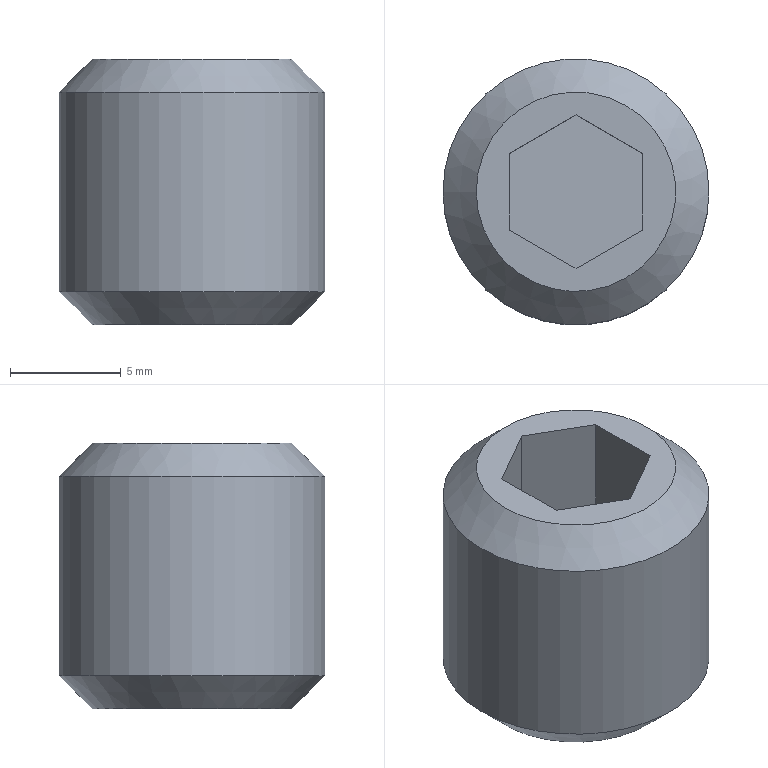Part | STEP file | gslz 2016.10.28-6_id326_x_t | 1 solid | 12 faces | box 12 x 12 x 12 mm | volume 1092 mm3 | plane 9 | cone 2 | cylinder 1 | commonest cylinder face diameters 12 x1
STEP:
#1=CARTESIAN_POINT('',(-76.95,184.,167.992));
#2=VERTEX_POINT('',#1);
#3=CARTESIAN_POINT('',(-82.95,184.,167.992));
#4=DIRECTION('',(0.,0.,-1.));
#5=DIRECTION('',(1.,0.,0.));
#6=AXIS2_PLACEMENT_3D('',#3,#4,#5);
#7=CIRCLE('',#6,6.);
#8=EDGE_CURVE('',#2,#2,#7,.T.);
#9=ORIENTED_EDGE('',*,*,#8,.F.);
#10=EDGE_LOOP('',(#9));
#11=FACE_BOUND('',#10,.T.);
#12=CARTESIAN_POINT('',(-88.95,184.,176.992));
#13=VERTEX_POINT('',#12);
#14=CARTESIAN_POINT('',(-82.95,184.,176.992));
#15=DIRECTION('',(0.,0.,1.));
#16=DIRECTION('',(-1.,0.,0.));
#17=AXIS2_PLACEMENT_3D('',#14,#15,#16);
#18=CIRCLE('',#17,6.);
#19=EDGE_CURVE('',#13,#13,#18,.T.);
#20=ORIENTED_EDGE('',*,*,#19,.F.);
#21=EDGE_LOOP('',(#20));
#22=FACE_BOUND('',#21,.T.);
#23=CARTESIAN_POINT('',(-82.95,184.,166.492));
#24=DIRECTION('',(0.,0.,1.));
#25=DIRECTION('',(1.,0.,0.));
#26=AXIS2_PLACEMENT_3D('',#23,#24,#25);
#27=CYLINDRICAL_SURFACE('',#26,6.);
#28=ADVANCED_FACE('',(#11,#22),#27,.T.);
#29=CARTESIAN_POINT('',(-78.45,184.,166.492));
#30=VERTEX_POINT('',#29);
#31=CARTESIAN_POINT('',(-82.95,184.,166.492));
#32=DIRECTION('',(0.,0.,1.));
#33=DIRECTION('',(1.,0.,0.));
#34=AXIS2_PLACEMENT_3D('',#31,#32,#33);
#35=CIRCLE('',#34,4.5);
#36=EDGE_CURVE('',#30,#30,#35,.T.);
#37=ORIENTED_EDGE('',*,*,#36,.F.);
#38=EDGE_LOOP('',(#37));
#39=FACE_OUTER_BOUND('',#38,.T.);
#40=CARTESIAN_POINT('',(-82.95,184.,166.492));
#41=DIRECTION('',(0.,0.,-1.));
#42=DIRECTION('',(-1.,0.,0.));
#43=AXIS2_PLACEMENT_3D('',#40,#41,#42);
#44=PLANE('',#43);
#45=ADVANCED_FACE('',(#39),#44,.T.);
#46=CARTESIAN_POINT('',(-87.45,184.,178.492));
#47=VERTEX_POINT('',#46);
#48=CARTESIAN_POINT('',(-82.95,184.,178.492));
#49=DIRECTION('',(0.,0.,-1.));
#50=DIRECTION('',(-1.,0.,0.));
#51=AXIS2_PLACEMENT_3D('',#48,#49,#50);
#52=CIRCLE('',#51,4.5);
#53=EDGE_CURVE('',#47,#47,#52,.T.);
#54=ORIENTED_EDGE('',*,*,#53,.F.);
#55=EDGE_LOOP('',(#54));
#56=FACE_BOUND('',#55,.T.);
#57=CARTESIAN_POINT('',(-85.95,182.268,178.492));
#58=VERTEX_POINT('',#57);
#59=CARTESIAN_POINT('',(-85.95,185.732,178.492));
#60=VERTEX_POINT('',#59);
#61=CARTESIAN_POINT('',(-85.95,179.959,178.492));
#62=DIRECTION('',(0.,1.,0.));
#63=VECTOR('',#62,1.);
#64=LINE('',#61,#63);
#65=EDGE_CURVE('',#58,#60,#64,.T.);
#66=ORIENTED_EDGE('',*,*,#65,.T.);
#67=CARTESIAN_POINT('',(-82.95,187.464,178.492));
#68=VERTEX_POINT('',#67);
#69=CARTESIAN_POINT('',(-87.95,184.577,178.492));
#70=DIRECTION('',(0.866,0.5,0.));
#71=VECTOR('',#70,1.);
#72=LINE('',#69,#71);
#73=EDGE_CURVE('',#60,#68,#72,.T.);
#74=ORIENTED_EDGE('',*,*,#73,.T.);
#75=CARTESIAN_POINT('',(-79.95,185.732,178.492));
#76=VERTEX_POINT('',#75);
#77=CARTESIAN_POINT('',(-84.95,188.619,178.492));
#78=DIRECTION('',(0.866,-0.5,0.));
#79=VECTOR('',#78,1.);
#80=LINE('',#77,#79);
#81=EDGE_CURVE('',#68,#76,#80,.T.);
#82=ORIENTED_EDGE('',*,*,#81,.T.);
#83=CARTESIAN_POINT('',(-79.95,182.268,178.492));
#84=VERTEX_POINT('',#83);
#85=CARTESIAN_POINT('',(-79.95,188.042,178.492));
#86=DIRECTION('',(0.,-1.,0.));
#87=VECTOR('',#86,1.);
#88=LINE('',#85,#87);
#89=EDGE_CURVE('',#76,#84,#88,.T.);
#90=ORIENTED_EDGE('',*,*,#89,.T.);
#91=CARTESIAN_POINT('',(-82.95,180.536,178.492));
#92=VERTEX_POINT('',#91);
#93=CARTESIAN_POINT('',(-77.95,183.423,178.492));
#94=DIRECTION('',(-0.866,-0.5,0.));
#95=VECTOR('',#94,1.);
#96=LINE('',#93,#95);
#97=EDGE_CURVE('',#84,#92,#96,.T.);
#98=ORIENTED_EDGE('',*,*,#97,.T.);
#99=CARTESIAN_POINT('',(-80.95,179.381,178.492));
#100=DIRECTION('',(-0.866,0.5,0.));
#101=VECTOR('',#100,1.);
#102=LINE('',#99,#101);
#103=EDGE_CURVE('',#92,#58,#102,.T.);
#104=ORIENTED_EDGE('',*,*,#103,.T.);
#105=EDGE_LOOP('',(#66,#74,#82,#90,#98,#104));
#106=FACE_BOUND('',#105,.T.);
#107=CARTESIAN_POINT('',(-82.95,184.,178.492));
#108=DIRECTION('',(0.,0.,1.));
#109=DIRECTION('',(1.,0.,0.));
#110=AXIS2_PLACEMENT_3D('',#107,#108,#109);
#111=PLANE('',#110);
#112=ADVANCED_FACE('',(#56,#106),#111,.T.);
#113=CARTESIAN_POINT('',(-85.95,182.268,172.492));
#114=VERTEX_POINT('',#113);
#115=CARTESIAN_POINT('',(-85.95,185.732,172.492));
#116=VERTEX_POINT('',#115);
#117=CARTESIAN_POINT('',(-85.95,179.959,172.492));
#118=DIRECTION('',(0.,1.,0.));
#119=VECTOR('',#118,1.);
#120=LINE('',#117,#119);
#121=EDGE_CURVE('',#114,#116,#120,.T.);
#122=ORIENTED_EDGE('',*,*,#121,.T.);
#123=CARTESIAN_POINT('',(-85.95,185.732,178.492));
#124=DIRECTION('',(0.,0.,-1.));
#125=VECTOR('',#124,1.);
#126=LINE('',#123,#125);
#127=EDGE_CURVE('',#60,#116,#126,.T.);
#128=ORIENTED_EDGE('',*,*,#127,.F.);
#129=ORIENTED_EDGE('',*,*,#65,.F.);
#130=CARTESIAN_POINT('',(-85.95,182.268,178.492));
#131=DIRECTION('',(0.,0.,-1.));
#132=VECTOR('',#131,1.);
#133=LINE('',#130,#132);
#134=EDGE_CURVE('',#58,#114,#133,.T.);
#135=ORIENTED_EDGE('',*,*,#134,.T.);
#136=EDGE_LOOP('',(#122,#128,#129,#135));
#137=FACE_OUTER_BOUND('',#136,.T.);
#138=CARTESIAN_POINT('',(-85.95,179.959,178.492));
#139=DIRECTION('',(1.,0.,0.));
#140=DIRECTION('',(0.,0.,-1.));
#141=AXIS2_PLACEMENT_3D('',#138,#139,#140);
#142=PLANE('',#141);
#143=ADVANCED_FACE('',(#137),#142,.T.);
#144=CARTESIAN_POINT('',(-82.95,187.464,172.492));
#145=VERTEX_POINT('',#144);
#146=CARTESIAN_POINT('',(-87.95,184.577,172.492));
#147=DIRECTION('',(0.866,0.5,0.));
#148=VECTOR('',#147,1.);
#149=LINE('',#146,#148);
#150=EDGE_CURVE('',#116,#145,#149,.T.);
#151=ORIENTED_EDGE('',*,*,#150,.T.);
#152=CARTESIAN_POINT('',(-82.95,187.464,178.492));
#153=DIRECTION('',(0.,0.,-1.));
#154=VECTOR('',#153,1.);
#155=LINE('',#152,#154);
#156=EDGE_CURVE('',#68,#145,#155,.T.);
#157=ORIENTED_EDGE('',*,*,#156,.F.);
#158=ORIENTED_EDGE('',*,*,#73,.F.);
#159=ORIENTED_EDGE('',*,*,#127,.T.);
#160=EDGE_LOOP('',(#151,#157,#158,#159));
#161=FACE_OUTER_BOUND('',#160,.T.);
#162=CARTESIAN_POINT('',(-87.95,184.577,178.492));
#163=DIRECTION('',(0.5,-0.866,0.));
#164=DIRECTION('',(-0.866,-0.5,0.));
#165=AXIS2_PLACEMENT_3D('',#162,#163,#164);
#166=PLANE('',#165);
#167=ADVANCED_FACE('',(#161),#166,.T.);
#168=CARTESIAN_POINT('',(-79.95,185.732,172.492));
#169=VERTEX_POINT('',#168);
#170=CARTESIAN_POINT('',(-84.95,188.619,172.492));
#171=DIRECTION('',(0.866,-0.5,0.));
#172=VECTOR('',#171,1.);
#173=LINE('',#170,#172);
#174=EDGE_CURVE('',#145,#169,#173,.T.);
#175=ORIENTED_EDGE('',*,*,#174,.T.);
#176=CARTESIAN_POINT('',(-79.95,185.732,178.492));
#177=DIRECTION('',(0.,0.,-1.));
#178=VECTOR('',#177,1.);
#179=LINE('',#176,#178);
#180=EDGE_CURVE('',#76,#169,#179,.T.);
#181=ORIENTED_EDGE('',*,*,#180,.F.);
#182=ORIENTED_EDGE('',*,*,#81,.F.);
#183=ORIENTED_EDGE('',*,*,#156,.T.);
#184=EDGE_LOOP('',(#175,#181,#182,#183));
#185=FACE_OUTER_BOUND('',#184,.T.);
#186=CARTESIAN_POINT('',(-84.95,188.619,178.492));
#187=DIRECTION('',(-0.5,-0.866,0.));
#188=DIRECTION('',(-0.866,0.5,0.));
#189=AXIS2_PLACEMENT_3D('',#186,#187,#188);
#190=PLANE('',#189);
#191=ADVANCED_FACE('',(#185),#190,.T.);
#192=CARTESIAN_POINT('',(-79.95,182.268,172.492));
#193=VERTEX_POINT('',#192);
#194=CARTESIAN_POINT('',(-79.95,188.042,172.492));
#195=DIRECTION('',(0.,-1.,0.));
#196=VECTOR('',#195,1.);
#197=LINE('',#194,#196);
#198=EDGE_CURVE('',#169,#193,#197,.T.);
#199=ORIENTED_EDGE('',*,*,#198,.T.);
#200=CARTESIAN_POINT('',(-79.95,182.268,178.492));
#201=DIRECTION('',(0.,0.,-1.));
#202=VECTOR('',#201,1.);
#203=LINE('',#200,#202);
#204=EDGE_CURVE('',#84,#193,#203,.T.);
#205=ORIENTED_EDGE('',*,*,#204,.F.);
#206=ORIENTED_EDGE('',*,*,#89,.F.);
#207=ORIENTED_EDGE('',*,*,#180,.T.);
#208=EDGE_LOOP('',(#199,#205,#206,#207));
#209=FACE_OUTER_BOUND('',#208,.T.);
#210=CARTESIAN_POINT('',(-79.95,188.042,178.492));
#211=DIRECTION('',(-1.,0.,0.));
#212=DIRECTION('',(0.,0.,1.));
#213=AXIS2_PLACEMENT_3D('',#210,#211,#212);
#214=PLANE('',#213);
#215=ADVANCED_FACE('',(#209),#214,.T.);
#216=CARTESIAN_POINT('',(-82.95,180.536,172.492));
#217=VERTEX_POINT('',#216);
#218=CARTESIAN_POINT('',(-77.95,183.423,172.492));
#219=DIRECTION('',(-0.866,-0.5,0.));
#220=VECTOR('',#219,1.);
#221=LINE('',#218,#220);
#222=EDGE_CURVE('',#193,#217,#221,.T.);
#223=ORIENTED_EDGE('',*,*,#222,.T.);
#224=CARTESIAN_POINT('',(-82.95,180.536,178.492));
#225=DIRECTION('',(0.,0.,-1.));
#226=VECTOR('',#225,1.);
#227=LINE('',#224,#226);
#228=EDGE_CURVE('',#92,#217,#227,.T.);
#229=ORIENTED_EDGE('',*,*,#228,.F.);
#230=ORIENTED_EDGE('',*,*,#97,.F.);
#231=ORIENTED_EDGE('',*,*,#204,.T.);
#232=EDGE_LOOP('',(#223,#229,#230,#231));
#233=FACE_OUTER_BOUND('',#232,.T.);
#234=CARTESIAN_POINT('',(-77.95,183.423,178.492));
#235=DIRECTION('',(-0.5,0.866,0.));
#236=DIRECTION('',(0.866,0.5,0.));
#237=AXIS2_PLACEMENT_3D('',#234,#235,#236);
#238=PLANE('',#237);
#239=ADVANCED_FACE('',(#233),#238,.T.);
#240=CARTESIAN_POINT('',(-80.95,179.381,172.492));
#241=DIRECTION('',(-0.866,0.5,0.));
#242=VECTOR('',#241,1.);
#243=LINE('',#240,#242);
#244=EDGE_CURVE('',#217,#114,#243,.T.);
#245=ORIENTED_EDGE('',*,*,#244,.T.);
#246=ORIENTED_EDGE('',*,*,#134,.F.);
#247=ORIENTED_EDGE('',*,*,#103,.F.);
#248=ORIENTED_EDGE('',*,*,#228,.T.);
#249=EDGE_LOOP('',(#245,#246,#247,#248));
#250=FACE_OUTER_BOUND('',#249,.T.);
#251=CARTESIAN_POINT('',(-80.95,179.381,178.492));
#252=DIRECTION('',(0.5,0.866,0.));
#253=DIRECTION('',(0.866,-0.5,0.));
#254=AXIS2_PLACEMENT_3D('',#251,#252,#253);
#255=PLANE('',#254);
#256=ADVANCED_FACE('',(#250),#255,.T.);
#257=ORIENTED_EDGE('',*,*,#121,.F.);
#258=ORIENTED_EDGE('',*,*,#244,.F.);
#259=ORIENTED_EDGE('',*,*,#222,.F.);
#260=ORIENTED_EDGE('',*,*,#198,.F.);
#261=ORIENTED_EDGE('',*,*,#174,.F.);
#262=ORIENTED_EDGE('',*,*,#150,.F.);
#263=EDGE_LOOP('',(#257,#258,#259,#260,#261,#262));
#264=FACE_OUTER_BOUND('',#263,.T.);
#265=CARTESIAN_POINT('',(-89.95,188.042,172.492));
#266=DIRECTION('',(0.,0.,1.));
#267=DIRECTION('',(1.,0.,0.));
#268=AXIS2_PLACEMENT_3D('',#265,#266,#267);
#269=PLANE('',#268);
#270=ADVANCED_FACE('',(#264),#269,.T.);
#271=ORIENTED_EDGE('',*,*,#8,.T.);
#272=EDGE_LOOP('',(#271));
#273=FACE_BOUND('',#272,.T.);
#274=ORIENTED_EDGE('',*,*,#36,.T.);
#275=EDGE_LOOP('',(#274));
#276=FACE_BOUND('',#275,.T.);
#277=CARTESIAN_POINT('',(-82.95,184.,166.492));
#278=DIRECTION('',(0.,0.,1.));
#279=DIRECTION('',(1.,0.,0.));
#280=AXIS2_PLACEMENT_3D('',#277,#278,#279);
#281=CONICAL_SURFACE('',#280,4.5,45.);
#282=ADVANCED_FACE('',(#273,#276),#281,.T.);
#283=ORIENTED_EDGE('',*,*,#53,.T.);
#284=EDGE_LOOP('',(#283));
#285=FACE_BOUND('',#284,.T.);
#286=ORIENTED_EDGE('',*,*,#19,.T.);
#287=EDGE_LOOP('',(#286));
#288=FACE_BOUND('',#287,.T.);
#289=CARTESIAN_POINT('',(-82.95,184.,176.992));
#290=DIRECTION('',(0.,0.,-1.));
#291=DIRECTION('',(-1.,0.,0.));
#292=AXIS2_PLACEMENT_3D('',#289,#290,#291);
#293=CONICAL_SURFACE('',#292,6.,45.);
#294=ADVANCED_FACE('',(#285,#288),#293,.T.);
#295=CLOSED_SHELL('',(#28,#45,#112,#143,#167,#191,#215,#239,#256,#270,#282,#294));
#296=MANIFOLD_SOLID_BREP('',#295);
#297=(LENGTH_UNIT()NAMED_UNIT(*)SI_UNIT(.MILLI.,.METRE.));
#298=UNCERTAINTY_MEASURE_WITH_UNIT(LENGTH_MEASURE(0.00002),#297,'','');
#299=(NAMED_UNIT(*)PLANE_ANGLE_UNIT()SI_UNIT($,.RADIAN.));
#300=PLANE_ANGLE_MEASURE_WITH_UNIT(PLANE_ANGLE_MEASURE(0.01745),#299);
#301=DIMENSIONAL_EXPONENTS(0.,0.,0.,0.,0.,0.,0.);
#302=(CONVERSION_BASED_UNIT('DEGREE',#300)NAMED_UNIT(#301)PLANE_ANGLE_UNIT());
#303=(NAMED_UNIT(*)SI_UNIT($,.STERADIAN.)SOLID_ANGLE_UNIT());
#304=(GEOMETRIC_REPRESENTATION_CONTEXT(3)GLOBAL_UNCERTAINTY_ASSIGNED_CONTEXT((#298))GLOBAL_UNIT_ASSIGNED_CONTEXT((#297,#302,#303))REPRESENTATION_CONTEXT('',''));
#305=ADVANCED_BREP_SHAPE_REPRESENTATION('',(#296),#304);